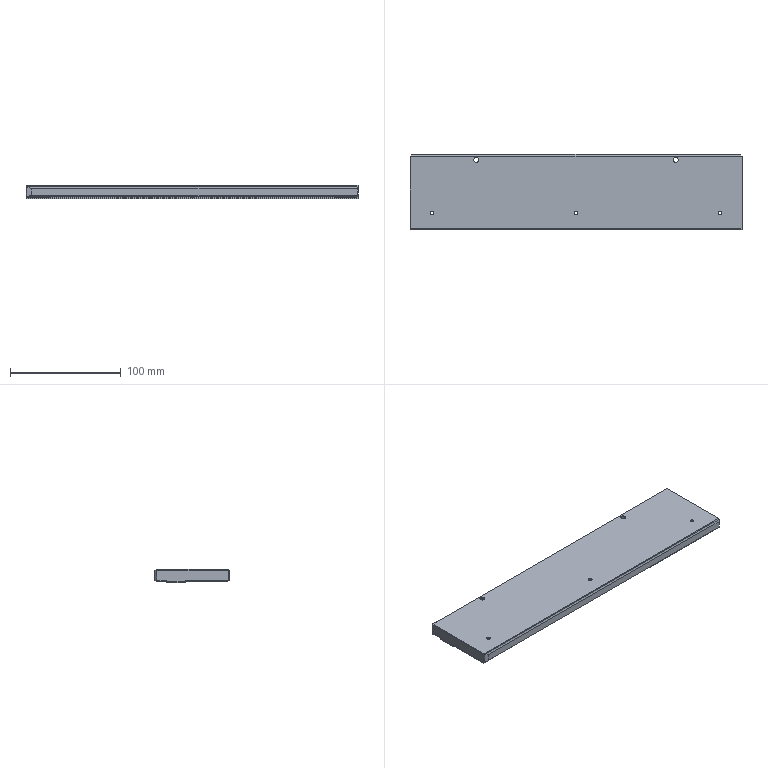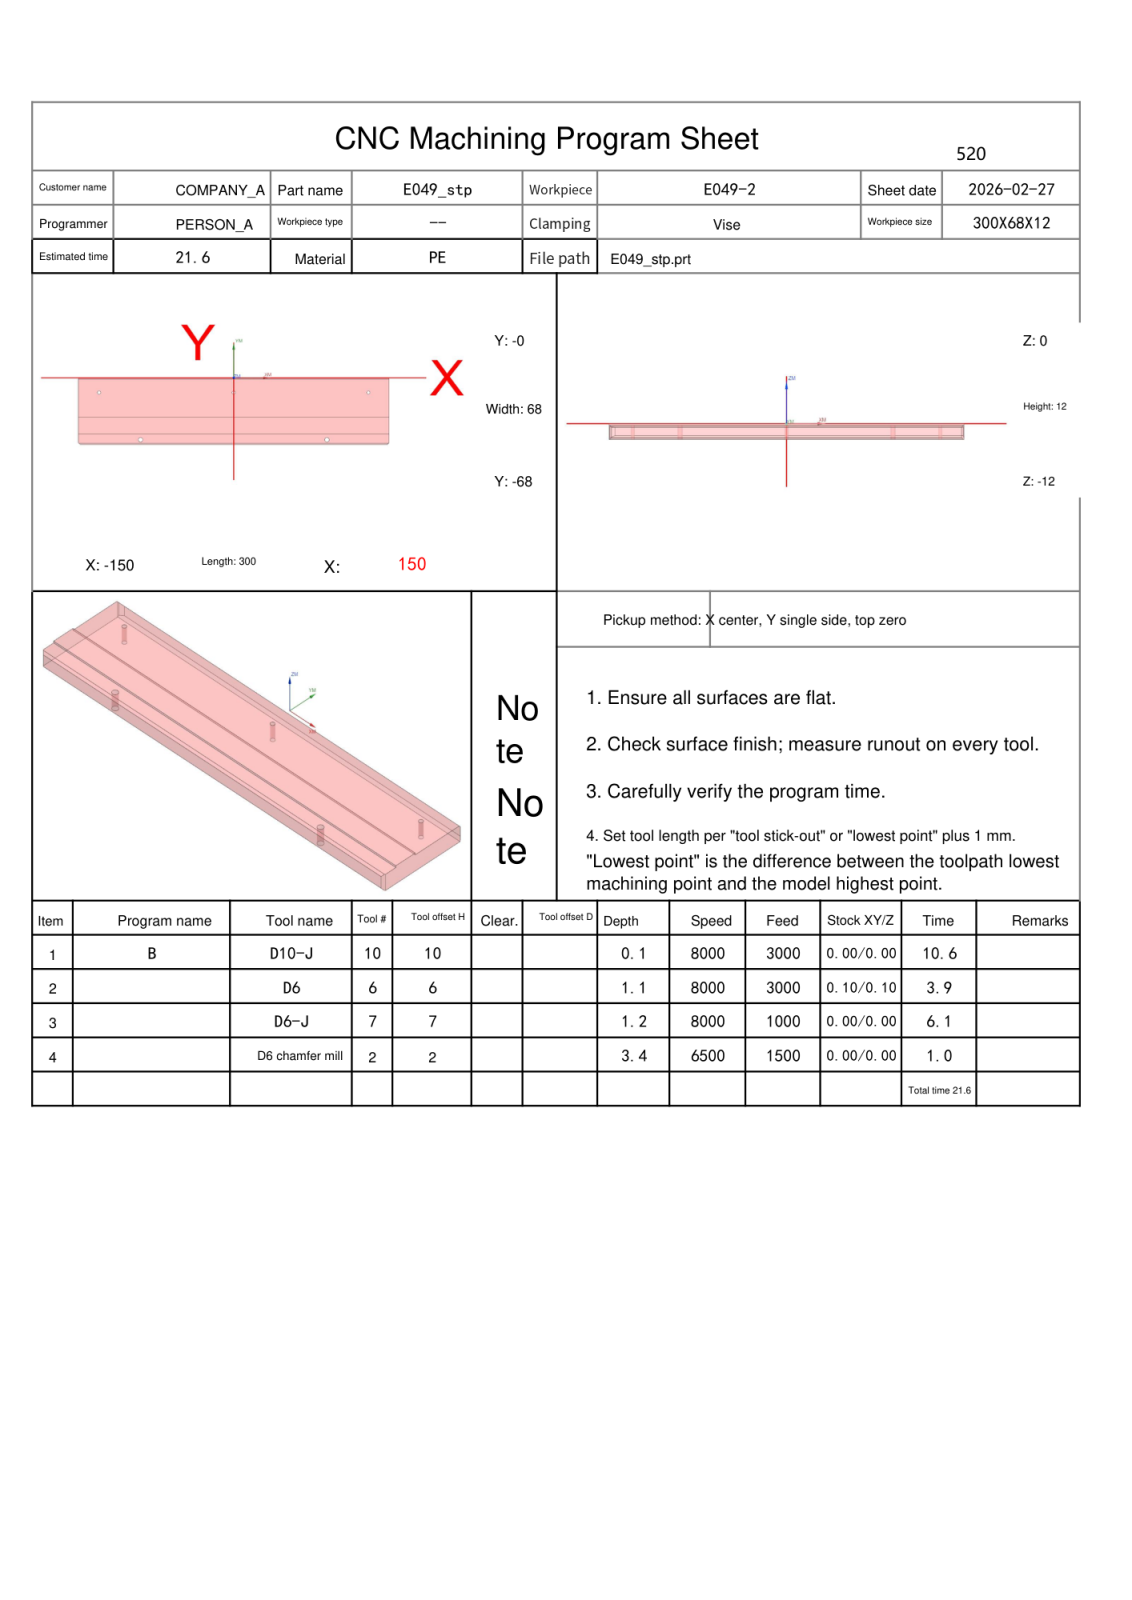NC program | NX | posted by the shop | part box 300 x 68 x 12 mm
Whole program:
%
O0001
(Machine time: 22.30 MIN)
(===Total Tool:4===)
(T10=D10-J  D=10.  R=0.   D-  H10 Z=0.    )
(T6=D6      D=6.   R=0.   D-  H06 Z=-1.1  )
(T7=D6-J    D=6.   R=0.   D7  H07 Z=-1.2  )
(T2=D6 chamfer mill   D=6.   R=0.   D-  H02 Z=-3.4  )
G80 G90 G17 G49 G40
G91 G28 Z0
M01
N1 T10 M06
(D10-J  D=10. R=0. H=10 ce=0.20 di=0.10)
G00 G90 G54 X-167. Y-16.7 M03 S8000
G43 H10 Z50.
M08
Z6.02
G01 Z4.02 F3000.
X-155. Y-4.7
X-145.593 Y4.707
G02 X-144.886 Y5. I.707 J-.707
G01 X-136.565
G02 X-136.166 Y4.6 I0.0 J-.4
X-136.283 Y4.317 I-.4 J0.0
G01 X-154.707 Y-14.107
G03 X-155. Y-14.814 I.707 J-.707
G01 Y-23.135
G03 X-154.6 Y-23.534 I.4 J0.0
X-154.317 Y-23.417 I0.0 J.4
G01 X-126.193 Y4.707
G02 X-125.486 Y5. I.707 J-.707
G01 X-117.165
G02 X-116.766 Y4.6 I0.0 J-.4
X-116.883 Y4.317 I-.4 J0.0
G01 X-154.707 Y-33.507
G03 X-155. Y-34.214 I.707 J-.707
G01 Y-42.535
G03 X-154.6 Y-42.934 I.4 J0.0
X-154.317 Y-42.817 I0.0 J.4
G01 X-106.793 Y4.707
G02 X-106.086 Y5. I.707 J-.707
G01 X-97.765
G02 X-97.366 Y4.6 I0.0 J-.4
X-97.483 Y4.317 I-.4 J0.0
G01 X-154.708 Y-52.908
G03 X-155. Y-53.614 I.708 J-.707
G01 Y-61.935
G03 X-154.6 Y-62.334 I.4 J0.0
X-154.317 Y-62.217 I0.0 J.4
G01 X-87.392 Y4.708
G02 X-86.686 Y5. I.707 J-.708
G01 X-78.365
G02 X-77.966 Y4.6 I0.0 J-.4
X-78.083 Y4.317 I-.4 J0.0
G01 X-154.717 Y-72.317
G03 X-154.834 Y-72.6 I.283 J-.283
X-154.435 Y-73. I.4 J0.0
G01 X-146.114
G03 X-145.408 Y-72.708 I-.001 J1.
G01 X-67.992 Y4.708
G02 X-67.286 Y5. I.707 J-.708
G01 X-58.965
G02 X-58.566 Y4.6 I0.0 J-.4
X-58.683 Y4.317 I-.4 J0.0
G01 X-135.317 Y-72.317
G03 X-135.434 Y-72.6 I.283 J-.283
X-135.035 Y-73. I.4 J0.0
G01 X-126.714
G03 X-126.008 Y-72.708 I-.001 J1.
G01 X-48.592 Y4.708
G02 X-47.886 Y5. I.707 J-.708
G01 X-39.565
G02 X-39.166 Y4.6 I0.0 J-.4
X-39.283 Y4.317 I-.4 J0.0
G01 X-115.917 Y-72.317
G03 X-116.034 Y-72.6 I.283 J-.283
X-115.635 Y-73. I.4 J0.0
G01 X-107.314
G03 X-106.608 Y-72.708 I-.001 J1.
G01 X-29.192 Y4.708
G02 X-28.486 Y5. I.707 J-.708
G01 X-20.165
G02 X-19.766 Y4.6 I0.0 J-.4
X-19.883 Y4.317 I-.4 J0.0
G01 X-96.517 Y-72.317
G03 X-96.634 Y-72.6 I.283 J-.283
X-96.235 Y-73. I.4 J0.0
G01 X-87.914
G03 X-87.208 Y-72.708 I-.001 J1.
G01 X-9.792 Y4.708
G02 X-9.086 Y5. I.707 J-.708
G01 X-.765
G02 X-.366 Y4.6 I0.0 J-.4
X-.483 Y4.317 I-.4 J0.0
G01 X-77.117 Y-72.317
G03 X-77.234 Y-72.6 I.283 J-.283
X-76.835 Y-73. I.4 J0.0
G01 X-68.514
G03 X-67.808 Y-72.708 I-.001 J1.
G01 X9.608 Y4.708
G02 X10.314 Y5. I.707 J-.708
G01 X18.635
G02 X19.034 Y4.6 I0.0 J-.4
X18.917 Y4.317 I-.4 J0.0
G01 X-57.717 Y-72.317
G03 X-57.834 Y-72.6 I.283 J-.283
X-57.435 Y-73. I.4 J0.0
G01 X-49.114
G03 X-48.408 Y-72.708 I-.001 J1.
G01 X29.008 Y4.708
G02 X29.714 Y5. I.707 J-.708
G01 X38.035
G02 X38.434 Y4.6 I0.0 J-.4
X38.317 Y4.317 I-.4 J0.0
G01 X-38.317 Y-72.317
G03 X-38.434 Y-72.6 I.283 J-.283
X-38.035 Y-73. I.4 J0.0
G01 X-29.714
G03 X-29.008 Y-72.708 I-.001 J1.
G01 X48.408 Y4.708
G02 X49.114 Y5. I.707 J-.708
G01 X57.435
G02 X57.834 Y4.6 I0.0 J-.4
X57.717 Y4.317 I-.4 J0.0
G01 X-18.917 Y-72.317
G03 X-19.034 Y-72.6 I.283 J-.283
X-18.635 Y-73. I.4 J0.0
G01 X-10.314
G03 X-9.608 Y-72.708 I-.001 J1.
G01 X67.808 Y4.708
G02 X68.514 Y5. I.707 J-.708
G01 X76.835
G02 X77.234 Y4.6 I0.0 J-.4
X77.117 Y4.317 I-.4 J0.0
G01 X.483 Y-72.317
G03 X.366 Y-72.6 I.283 J-.283
X.765 Y-73. I.4 J0.0
G01 X9.086
G03 X9.792 Y-72.708 I-.001 J1.
G01 X87.208 Y4.708
G02 X87.914 Y5. I.707 J-.708
G01 X96.235
G02 X96.634 Y4.6 I0.0 J-.4
X96.517 Y4.317 I-.4 J0.0
G01 X19.883 Y-72.317
G03 X19.766 Y-72.6 I.283 J-.283
X20.165 Y-73. I.4 J0.0
G01 X28.486
G03 X29.192 Y-72.708 I-.001 J1.
G01 X106.608 Y4.708
G02 X107.314 Y5. I.707 J-.708
G01 X115.635
G02 X116.034 Y4.6 I0.0 J-.4
X115.917 Y4.317 I-.4 J0.0
G01 X39.283 Y-72.317
G03 X39.166 Y-72.6 I.283 J-.283
X39.565 Y-73. I.4 J0.0
G01 X47.886
G03 X48.592 Y-72.708 I-.001 J1.
G01 X126.008 Y4.708
G02 X126.714 Y5. I.707 J-.708
G01 X135.035
G02 X135.434 Y4.6 I0.0 J-.4
X135.317 Y4.317 I-.4 J0.0
G01 X58.683 Y-72.317
G03 X58.566 Y-72.6 I.283 J-.283
X58.965 Y-73. I.4 J0.0
G01 X67.286
G03 X67.992 Y-72.708 I-.001 J1.
G01 X145.408 Y4.708
G02 X146.114 Y5. I.707 J-.708
G01 X154.435
G02 X154.834 Y4.6 I0.0 J-.4
X154.717 Y4.317 I-.4 J0.0
G01 X78.083 Y-72.317
G03 X77.966 Y-72.6 I.283 J-.283
X78.365 Y-73. I.4 J0.0
G01 X86.686
G03 X87.392 Y-72.708 I-.001 J1.
G01 X154.317 Y-5.783
G02 X154.6 Y-5.666 I.283 J-.283
X155. Y-6.065 I0.0 J-.4
G01 Y-14.386
G02 X154.708 Y-15.092 I-1. J.001
G01 X97.483 Y-72.317
G03 X97.366 Y-72.6 I.283 J-.283
X97.765 Y-73. I.4 J0.0
G01 X106.086
G03 X106.792 Y-72.708 I-.001 J1.
G01 X154.317 Y-25.183
G02 X154.6 Y-25.066 I.283 J-.283
X155. Y-25.465 I0.0 J-.4
G01 Y-33.786
G02 X154.707 Y-34.493 I-1. J.001
G01 X116.883 Y-72.317
G03 X116.766 Y-72.6 I.283 J-.283
X117.165 Y-73. I.4 J0.0
G01 X125.486
G03 X126.193 Y-72.707 I0.0 J1.
G01 X154.317 Y-44.583
G02 X154.6 Y-44.466 I.283 J-.283
X155. Y-44.865 I0.0 J-.4
G01 Y-53.186
G02 X154.707 Y-53.893 I-1. J0.0
G01 X136.283 Y-72.317
G03 X136.166 Y-72.6 I.283 J-.283
X136.565 Y-73. I.4 J0.0
G01 X144.886
G03 X145.593 Y-72.707 I0.0 J1.
G01 X155. Y-63.3
X167. Y-51.3
Z6.02
G00 Z8.
X-167. Y-16.7
Z5.04
G01 Z3.04
X-155. Y-4.7
X-145.593 Y4.707
G02 X-144.886 Y5. I.707 J-.707
G01 X-136.565
G02 X-136.166 Y4.6 I0.0 J-.4
X-136.283 Y4.317 I-.4 J0.0
G01 X-154.707 Y-14.107
G03 X-155. Y-14.814 I.707 J-.707
G01 Y-23.135
G03 X-154.6 Y-23.534 I.4 J0.0
X-154.317 Y-23.417 I0.0 J.4
G01 X-126.193 Y4.707
G02 X-125.486 Y5. I.707 J-.707
G01 X-117.165
G02 X-116.766 Y4.6 I0.0 J-.4
X-116.883 Y4.317 I-.4 J0.0
G01 X-154.707 Y-33.507
G03 X-155. Y-34.214 I.707 J-.707
G01 Y-42.535
G03 X-154.6 Y-42.934 I.4 J0.0
X-154.317 Y-42.817 I0.0 J.4
G01 X-106.793 Y4.707
G02 X-106.086 Y5. I.707 J-.707
G01 X-97.765
G02 X-97.366 Y4.6 I0.0 J-.4
X-97.483 Y4.317 I-.4 J0.0
G01 X-154.708 Y-52.908
G03 X-155. Y-53.614 I.708 J-.707
G01 Y-61.935
G03 X-154.6 Y-62.334 I.4 J0.0
X-154.317 Y-62.217 I0.0 J.4
G01 X-87.392 Y4.708
G02 X-86.686 Y5. I.707 J-.708
G01 X-78.365
G02 X-77.966 Y4.6 I0.0 J-.4
X-78.083 Y4.317 I-.4 J0.0
G01 X-154.717 Y-72.317
G03 X-154.834 Y-72.6 I.283 J-.283
X-154.435 Y-73. I.4 J0.0
G01 X-146.114
G03 X-145.408 Y-72.708 I-.001 J1.
G01 X-67.992 Y4.708
G02 X-67.286 Y5. I.707 J-.708
G01 X-58.965
G02 X-58.566 Y4.6 I0.0 J-.4
X-58.683 Y4.317 I-.4 J0.0
G01 X-135.317 Y-72.317
G03 X-135.434 Y-72.6 I.283 J-.283
X-135.035 Y-73. I.4 J0.0
G01 X-126.714
G03 X-126.008 Y-72.708 I-.001 J1.
G01 X-48.592 Y4.708
G02 X-47.886 Y5. I.707 J-.708
G01 X-39.565
G02 X-39.166 Y4.6 I0.0 J-.4
X-39.283 Y4.317 I-.4 J0.0
G01 X-115.917 Y-72.317
G03 X-116.034 Y-72.6 I.283 J-.283
X-115.635 Y-73. I.4 J0.0
G01 X-107.314
G03 X-106.608 Y-72.708 I-.001 J1.
G01 X-29.192 Y4.708
G02 X-28.486 Y5. I.707 J-.708
G01 X-20.165
G02 X-19.766 Y4.6 I0.0 J-.4
X-19.883 Y4.317 I-.4 J0.0
G01 X-96.517 Y-72.317
G03 X-96.634 Y-72.6 I.283 J-.283
X-96.235 Y-73. I.4 J0.0
G01 X-87.914
G03 X-87.208 Y-72.708 I-.001 J1.
G01 X-9.792 Y4.708
G02 X-9.086 Y5. I.707 J-.708
G01 X-.765
G02 X-.366 Y4.6 I0.0 J-.4
X-.483 Y4.317 I-.4 J0.0
G01 X-77.117 Y-72.317
G03 X-77.234 Y-72.6 I.283 J-.283
X-76.835 Y-73. I.4 J0.0
G01 X-68.514
G03 X-67.808 Y-72.708 I-.001 J1.
G01 X9.608 Y4.708
G02 X10.314 Y5. I.707 J-.708
G01 X18.635
G02 X19.034 Y4.6 I0.0 J-.4
X18.917 Y4.317 I-.4 J0.0
G01 X-57.717 Y-72.317
G03 X-57.834 Y-72.6 I.283 J-.283
X-57.435 Y-73. I.4 J0.0
G01 X-49.114
G03 X-48.408 Y-72.708 I-.001 J1.
G01 X29.008 Y4.708
G02 X29.714 Y5. I.707 J-.708
G01 X38.035
G02 X38.434 Y4.6 I0.0 J-.4
X38.317 Y4.317 I-.4 J0.0
G01 X-38.317 Y-72.317
G03 X-38.434 Y-72.6 I.283 J-.283
X-38.035 Y-73. I.4 J0.0
G01 X-29.714
G03 X-29.008 Y-72.708 I-.001 J1.
G01 X48.408 Y4.708
G02 X49.114 Y5. I.707 J-.708
G01 X57.435
G02 X57.834 Y4.6 I0.0 J-.4
X57.717 Y4.317 I-.4 J0.0
G01 X-18.917 Y-72.317
G03 X-19.034 Y-72.6 I.283 J-.283
X-18.635 Y-73. I.4 J0.0
G01 X-10.314
G03 X-9.608 Y-72.708 I-.001 J1.
G01 X67.808 Y4.708
G02 X68.514 Y5. I.707 J-.708
G01 X76.835
G02 X77.234 Y4.6 I0.0 J-.4
X77.117 Y4.317 I-.4 J0.0
G01 X.483 Y-72.317
G03 X.366 Y-72.6 I.283 J-.283
X.765 Y-73. I.4 J0.0
G01 X9.086
G03 X9.792 Y-72.708 I-.001 J1.
G01 X87.208 Y4.708
G02 X87.914 Y5. I.707 J-.708
G01 X96.235
G02 X96.634 Y4.6 I0.0 J-.4
X96.517 Y4.317 I-.4 J0.0
G01 X19.883 Y-72.317
G03 X19.766 Y-72.6 I.283 J-.283
X20.165 Y-73. I.4 J0.0
G01 X28.486
G03 X29.192 Y-72.708 I-.001 J1.
G01 X106.608 Y4.708
G02 X107.314 Y5. I.707 J-.708
G01 X115.635
G02 X116.034 Y4.6 I0.0 J-.4
X115.917 Y4.317 I-.4 J0.0
G01 X39.283 Y-72.317
G03 X39.166 Y-72.6 I.283 J-.283
X39.565 Y-73. I.4 J0.0
G01 X47.886
G03 X48.592 Y-72.708 I-.001 J1.
G01 X126.008 Y4.708
G02 X126.714 Y5. I.707 J-.708
G01 X135.035
G02 X135.434 Y4.6 I0.0 J-.4
X135.317 Y4.317 I-.4 J0.0
G01 X58.683 Y-72.317
G03 X58.566 Y-72.6 I.283 J-.283
X58.965 Y-73. I.4 J0.0
G01 X67.286
G03 X67.992 Y-72.708 I-.001 J1.
G01 X145.408 Y4.708
G02 X146.114 Y5. I.707 J-.708
G01 X154.435
G02 X154.834 Y4.6 I0.0 J-.4
X154.717 Y4.317 I-.4 J0.0
G01 X78.083 Y-72.317
G03 X77.966 Y-72.6 I.283 J-.283
X78.365 Y-73. I.4 J0.0
G01 X86.686
G03 X87.392 Y-72.708 I-.001 J1.
G01 X154.317 Y-5.783
G02 X154.6 Y-5.666 I.283 J-.283
X155. Y-6.065 I0.0 J-.4
G01 Y-14.386
G02 X154.708 Y-15.092 I-1. J.001
G01 X97.483 Y-72.317
G03 X97.366 Y-72.6 I.283 J-.283
X97.765 Y-73. I.4 J0.0
G01 X106.086
G03 X106.792 Y-72.708 I-.001 J1.
G01 X154.317 Y-25.183
G02 X154.6 Y-25.066 I.283 J-.283
X155. Y-25.465 I0.0 J-.4
G01 Y-33.786
G02 X154.707 Y-34.493 I-1. J.001
G01 X116.883 Y-72.317
G03 X116.766 Y-72.6 I.283 J-.283
X117.165 Y-73. I.4 J0.0
G01 X125.486
G03 X126.193 Y-72.707 I0.0 J1.
G01 X154.317 Y-44.583
G02 X154.6 Y-44.466 I.283 J-.283
X155. Y-44.865 I0.0 J-.4
G01 Y-53.186
G02 X154.707 Y-53.893 I-1. J0.0
G01 X136.283 Y-72.317
G03 X136.166 Y-72.6 I.283 J-.283
X136.565 Y-73. I.4 J0.0
G01 X144.886
G03 X145.593 Y-72.707 I0.0 J1.
G01 X155. Y-63.3
X167. Y-51.3
Z5.04
G00 Z7.02
X-167. Y-16.7
Z4.06
G01 Z2.06
X-155. Y-4.7
X-145.593 Y4.707
G02 X-144.886 Y5. I.707 J-.707
G01 X-136.565
G02 X-136.166 Y4.6 I0.0 J-.4
X-136.283 Y4.317 I-.4 J0.0
G01 X-154.707 Y-14.107
G03 X-155. Y-14.814 I.707 J-.707
G01 Y-23.135
G03 X-154.6 Y-23.534 I.4 J0.0
X-154.317 Y-23.417 I0.0 J.4
G01 X-126.193 Y4.707
G02 X-125.486 Y5. I.707 J-.707
G01 X-117.165
G02 X-116.766 Y4.6 I0.0 J-.4
X-116.883 Y4.317 I-.4 J0.0
G01 X-154.707 Y-33.507
G03 X-155. Y-34.214 I.707 J-.707
G01 Y-42.535
G03 X-154.6 Y-42.934 I.4 J0.0
X-154.317 Y-42.817 I0.0 J.4
G01 X-106.793 Y4.707
G02 X-106.086 Y5. I.707 J-.707
G01 X-97.765
G02 X-97.366 Y4.6 I0.0 J-.4
X-97.483 Y4.317 I-.4 J0.0
G01 X-154.708 Y-52.908
G03 X-155. Y-53.614 I.708 J-.707
G01 Y-61.935
G03 X-154.6 Y-62.334 I.4 J0.0
X-154.317 Y-62.217 I0.0 J.4
G01 X-87.392 Y4.708
G02 X-86.686 Y5. I.707 J-.708
G01 X-78.365
G02 X-77.966 Y4.6 I0.0 J-.4
X-78.083 Y4.317 I-.4 J0.0
G01 X-154.717 Y-72.317
G03 X-154.834 Y-72.6 I.283 J-.283
X-154.435 Y-73. I.4 J0.0
G01 X-146.114
G03 X-145.408 Y-72.708 I-.001 J1.
G01 X-67.992 Y4.708
G02 X-67.286 Y5. I.707 J-.708
G01 X-58.965
G02 X-58.566 Y4.6 I0.0 J-.4
X-58.683 Y4.317 I-.4 J0.0
G01 X-135.317 Y-72.317
G03 X-135.434 Y-72.6 I.283 J-.283
X-135.035 Y-73. I.4 J0.0
G01 X-126.714
G03 X-126.008 Y-72.708 I-.001 J1.
G01 X-48.592 Y4.708
G02 X-47.886 Y5. I.707 J-.708
G01 X-39.565
G02 X-39.166 Y4.6 I0.0 J-.4
X-39.283 Y4.317 I-.4 J0.0
G01 X-115.917 Y-72.317
G03 X-116.034 Y-72.6 I.283 J-.283
X-115.635 Y-73. I.4 J0.0
G01 X-107.314
G03 X-106.608 Y-72.708 I-.001 J1.
G01 X-29.192 Y4.708
G02 X-28.486 Y5. I.707 J-.708
G01 X-20.165
G02 X-19.766 Y4.6 I0.0 J-.4
X-19.883 Y4.317 I-.4 J0.0
G01 X-96.517 Y-72.317
G03 X-96.634 Y-72.6 I.283 J-.283
X-96.235 Y-73. I.4 J0.0
G01 X-87.914
G03 X-87.208 Y-72.708 I-.001 J1.
G01 X-9.792 Y4.708
G02 X-9.086 Y5. I.707 J-.708
G01 X-.765
G02 X-.366 Y4.6 I0.0 J-.4
X-.483 Y4.317 I-.4 J0.0
G01 X-77.117 Y-72.317
G03 X-77.234 Y-72.6 I.283 J-.283
X-76.835 Y-73. I.4 J0.0
G01 X-68.514
G03 X-67.808 Y-72.708 I-.001 J1.
G01 X9.608 Y4.708
G02 X10.314 Y5. I.707 J-.708
G01 X18.635
G02 X19.034 Y4.6 I0.0 J-.4
X18.917 Y4.317 I-.4 J0.0
G01 X-57.717 Y-72.317
G03 X-57.834 Y-72.6 I.283 J-.283
X-57.435 Y-73. I.4 J0.0
G01 X-49.114
G03 X-48.408 Y-72.708 I-.001 J1.
G01 X29.008 Y4.708
G02 X29.714 Y5. I.707 J-.708
G01 X38.035
G02 X38.434 Y4.6 I0.0 J-.4
X38.317 Y4.317 I-.4 J0.0
G01 X-38.317 Y-72.317
G03 X-38.434 Y-72.6 I.283 J-.283
X-38.035 Y-73. I.4 J0.0
G01 X-29.714
G03 X-29.008 Y-72.708 I-.001 J1.
G01 X48.408 Y4.708
G02 X49.114 Y5. I.707 J-.708
G01 X57.435
G02 X57.834 Y4.6 I0.0 J-.4
X57.717 Y4.317 I-.4 J0.0
G01 X-18.917 Y-72.317
G03 X-19.034 Y-72.6 I.283 J-.283
X-18.635 Y-73. I.4 J0.0
G01 X-10.314
G03 X-9.608 Y-72.708 I-.001 J1.
G01 X67.808 Y4.708
G02 X68.514 Y5. I.707 J-.708
G01 X76.835
G02 X77.234 Y4.6 I0.0 J-.4
X77.117 Y4.317 I-.4 J0.0
G01 X.483 Y-72.317
G03 X.366 Y-72.6 I.283 J-.283
X.765 Y-73. I.4 J0.0
G01 X9.086
G03 X9.792 Y-72.708 I-.001 J1.
G01 X87.208 Y4.708
G02 X87.914 Y5. I.707 J-.708
G01 X96.235
G02 X96.634 Y4.6 I0.0 J-.4
X96.517 Y4.317 I-.4 J0.0
G01 X19.883 Y-72.317
G03 X19.766 Y-72.6 I.283 J-.283
X20.165 Y-73. I.4 J0.0
G01 X28.486
G03 X29.192 Y-72.708 I-.001 J1.
G01 X106.608 Y4.708
G02 X107.314 Y5. I.707 J-.708
G01 X115.635
G02 X116.034 Y4.6 I0.0 J-.4
X115.917 Y4.317 I-.4 J0.0
G01 X39.283 Y-72.317
G03 X39.166 Y-72.6 I.283 J-.283
X39.565 Y-73. I.4 J0.0
G01 X47.886
G03 X48.592 Y-72.708 I-.001 J1.
G01 X126.008 Y4.708
G02 X126.714 Y5. I.707 J-.708
G01 X135.035
G02 X135.434 Y4.6 I0.0 J-.4
X135.317 Y4.317 I-.4 J0.0
G01 X58.683 Y-72.317
G03 X58.566 Y-72.6 I.283 J-.283
X58.965 Y-73. I.4 J0.0
G01 X67.286
G03 X67.992 Y-72.708 I-.001 J1.
G01 X145.408 Y4.708
G02 X146.114 Y5. I.707 J-.708
G01 X154.435
G02 X154.834 Y4.6 I0.0 J-.4
X154.717 Y4.317 I-.4 J0.0
G01 X78.083 Y-72.317
G03 X77.966 Y-72.6 I.283 J-.283
X78.365 Y-73. I.4 J0.0
G01 X86.686
G03 X87.392 Y-72.708 I-.001 J1.
G01 X154.317 Y-5.783
G02 X154.6 Y-5.666 I.283 J-.283
X155. Y-6.065 I0.0 J-.4
G01 Y-14.386
G02 X154.708 Y-15.092 I-1. J.001
G01 X97.483 Y-72.317
G03 X97.366 Y-72.6 I.283 J-.283
X97.765 Y-73. I.4 J0.0
G01 X106.086
G03 X106.792 Y-72.708 I-.001 J1.
G01 X154.317 Y-25.183
G02 X154.6 Y-25.066 I.283 J-.283
X155. Y-25.465 I0.0 J-.4
G01 Y-33.786
G02 X154.707 Y-34.493 I-1. J.001
G01 X116.883 Y-72.317
G03 X116.766 Y-72.6 I.283 J-.283
X117.165 Y-73. I.4 J0.0
G01 X125.486
G03 X126.193 Y-72.707 I0.0 J1.
G01 X154.317 Y-44.583
G02 X154.6 Y-44.466 I.283 J-.283
X155. Y-44.865 I0.0 J-.4
G01 Y-53.186
G02 X154.707 Y-53.893 I-1. J0.0
G01 X136.283 Y-72.317
G03 X136.166 Y-72.6 I.283 J-.283
X136.565 Y-73. I.4 J0.0
G01 X144.886
G03 X145.593 Y-72.707 I0.0 J1.
G01 X155. Y-63.3
X167. Y-51.3
Z4.06
G00 Z6.04
X-167. Y-16.7
Z3.08
G01 Z1.08
X-155. Y-4.7
X-145.593 Y4.707
G02 X-144.886 Y5. I.707 J-.707
G01 X-136.565
G02 X-136.166 Y4.6 I0.0 J-.4
X-136.283 Y4.317 I-.4 J0.0
G01 X-154.707 Y-14.107
G03 X-155. Y-14.814 I.707 J-.707
G01 Y-23.135
G03 X-154.6 Y-23.534 I.4 J0.0
X-154.317 Y-23.417 I0.0 J.4
G01 X-126.193 Y4.707
G02 X-125.486 Y5. I.707 J-.707
G01 X-117.165
G02 X-116.766 Y4.6 I0.0 J-.4
X-116.883 Y4.317 I-.4 J0.0
G01 X-154.707 Y-33.507
G03 X-155. Y-34.214 I.707 J-.707
G01 Y-42.535
G03 X-154.6 Y-42.934 I.4 J0.0
X-154.317 Y-42.817 I0.0 J.4
G01 X-106.793 Y4.707
G02 X-106.086 Y5. I.707 J-.707
G01 X-97.765
G02 X-97.366 Y4.6 I0.0 J-.4
X-97.483 Y4.317 I-.4 J0.0
G01 X-154.708 Y-52.908
G03 X-155. Y-53.614 I.708 J-.707
G01 Y-61.935
G03 X-154.6 Y-62.334 I.4 J0.0
X-154.317 Y-62.217 I0.0 J.4
G01 X-87.392 Y4.708
G02 X-86.686 Y5. I.707 J-.708
G01 X-78.365
G02 X-77.966 Y4.6 I0.0 J-.4
X-78.083 Y4.317 I-.4 J0.0
G01 X-154.717 Y-72.317
G03 X-154.834 Y-72.6 I.283 J-.283
X-154.435 Y-73. I.4 J0.0
G01 X-146.114
G03 X-145.408 Y-72.708 I-.001 J1.
G01 X-67.992 Y4.708
G02 X-67.286 Y5. I.707 J-.708
G01 X-58.965
G02 X-58.566 Y4.6 I0.0 J-.4
X-58.683 Y4.317 I-.4 J0.0
G01 X-135.317 Y-72.317
G03 X-135.434 Y-72.6 I.283 J-.283
X-135.035 Y-73. I.4 J0.0
G01 X-126.714
G03 X-126.008 Y-72.708 I-.001 J1.
G01 X-48.592 Y4.708
G02 X-47.886 Y5. I.707 J-.708
G01 X-39.565
G02 X-39.166 Y4.6 I0.0 J-.4
X-39.283 Y4.317 I-.4 J0.0
G01 X-115.917 Y-72.317
G03 X-116.034 Y-72.6 I.283 J-.283
X-115.635 Y-73. I.4 J0.0
G01 X-107.314
G03 X-106.608 Y-72.708 I-.001 J1.
G01 X-29.192 Y4.708
G02 X-28.486 Y5. I.707 J-.708
G01 X-20.165
G02 X-19.766 Y4.6 I0.0 J-.4
X-19.883 Y4.317 I-.4 J0.0
G01 X-96.517 Y-72.317
G03 X-96.634 Y-72.6 I.283 J-.283
X-96.235 Y-73. I.4 J0.0
G01 X-87.914
G03 X-87.208 Y-72.708 I-.001 J1.
G01 X-9.792 Y4.708
G02 X-9.086 Y5. I.707 J-.708
G01 X-.765
G02 X-.366 Y4.6 I0.0 J-.4
X-.483 Y4.317 I-.4 J0.0
G01 X-77.117 Y-72.317
G03 X-77.234 Y-72.6 I.283 J-.283
X-76.835 Y-73. I.4 J0.0
G01 X-68.514
G03 X-67.808 Y-72.708 I-.001 J1.
G01 X9.608 Y4.708
G02 X10.314 Y5. I.707 J-.708
G01 X18.635
G02 X19.034 Y4.6 I0.0 J-.4
X18.917 Y4.317 I-.4 J0.0
G01 X-57.717 Y-72.317
G03 X-57.834 Y-72.6 I.283 J-.283
X-57.435 Y-73. I.4 J0.0
G01 X-49.114
G03 X-48.408 Y-72.708 I-.001 J1.
G01 X29.008 Y4.708
G02 X29.714 Y5. I.707 J-.708
G01 X38.035
G02 X38.434 Y4.6 I0.0 J-.4
X38.317 Y4.317 I-.4 J0.0
G01 X-38.317 Y-72.317
G03 X-38.434 Y-72.6 I.283 J-.283
X-38.035 Y-73. I.4 J0.0
G01 X-29.714
G03 X-29.008 Y-72.708 I-.001 J1.
G01 X48.408 Y4.708
G02 X49.114 Y5. I.707 J-.708
G01 X57.435
G02 X57.834 Y4.6 I0.0 J-.4
X57.717 Y4.317 I-.4 J0.0
G01 X-18.917 Y-72.317
G03 X-19.034 Y-72.6 I.283 J-.283
X-18.635 Y-73. I.4 J0.0
G01 X-10.314
G03 X-9.608 Y-72.708 I-.001 J1.
G01 X67.808 Y4.708
G02 X68.514 Y5. I.707 J-.708
G01 X76.835
G02 X77.234 Y4.6 I0.0 J-.4
X77.117 Y4.317 I-.4 J0.0
G01 X.483 Y-72.317
G03 X.366 Y-72.6 I.283 J-.283
X.765 Y-73. I.4 J0.0
G01 X9.086
G03 X9.792 Y-72.708 I-.001 J1.
G01 X87.208 Y4.708
G02 X87.914 Y5. I.707 J-.708
G01 X96.235
G02 X96.634 Y4.6 I0.0 J-.4
X96.517 Y4.317 I-.4 J0.0
G01 X19.883 Y-72.317
G03 X19.766 Y-72.6 I.283 J-.283
X20.165 Y-73. I.4 J0.0
G01 X28.486
G03 X29.192 Y-72.708 I-.001 J1.
G01 X106.608 Y4.708
G02 X107.314 Y5. I.707 J-.708
G01 X115.635
G02 X116.034 Y4.6 I0.0 J-.4
X115.917 Y4.317 I-.4 J0.0
G01 X39.283 Y-72.317
G03 X39.166 Y-72.6 I.283 J-.283
X39.565 Y-73. I.4 J0.0
G01 X47.886
G03 X48.592 Y-72.708 I-.001 J1.
G01 X126.008 Y4.708
G02 X126.714 Y5. I.707 J-.708
G01 X135.035
G02 X135.434 Y4.6 I0.0 J-.4
X135.317 Y4.317 I-.4 J0.0
G01 X58.683 Y-72.317
G03 X58.566 Y-72.6 I.283 J-.283
X58.965 Y-73. I.4 J0.0
G01 X67.286
G03 X67.992 Y-72.708 I-.001 J1.
G01 X145.408 Y4.708
G02 X146.114 Y5. I.707 J-.708
G01 X154.435
G02 X154.834 Y4.6 I0.0 J-.4
X154.717 Y4.317 I-.4 J0.0
G01 X78.083 Y-72.317
G03 X77.966 Y-72.6 I.283 J-.283
X78.365 Y-73. I.4 J0.0
G01 X86.686
G03 X87.392 Y-72.708 I-.001 J1.
G01 X154.317 Y-5.783
G02 X154.6 Y-5.666 I.283 J-.283
X155. Y-6.065 I0.0 J-.4
G01 Y-14.386
G02 X154.708 Y-15.092 I-1. J.001
G01 X97.483 Y-72.317
G03 X97.366 Y-72.6 I.283 J-.283
X97.765 Y-73. I.4 J0.0
G01 X106.086
G03 X106.792 Y-72.708 I-.001 J1.
G01 X154.317 Y-25.183
G02 X154.6 Y-25.066 I.283 J-.283
X155. Y-25.465 I0.0 J-.4
G01 Y-33.786
G02 X154.707 Y-34.493 I-1. J.001
G01 X116.883 Y-72.317
G03 X116.766 Y-72.6 I.283 J-.283
X117.165 Y-73. I.4 J0.0
G01 X125.486
G03 X126.193 Y-72.707 I0.0 J1.
G01 X154.317 Y-44.583
G02 X154.6 Y-44.466 I.283 J-.283
X155. Y-44.865 I0.0 J-.4
G01 Y-53.186
G02 X154.707 Y-53.893 I-1. J0.0
G01 X136.283 Y-72.317
G03 X136.166 Y-72.6 I.283 J-.283
X136.565 Y-73. I.4 J0.0
G01 X144.886
G03 X145.593 Y-72.707 I0.0 J1.
G01 X155. Y-63.3
X167. Y-51.3
Z3.08
G00 Z5.06
X-167. Y-16.7
Z2.1
G01 Z.1
X-155. Y-4.7
X-145.593 Y4.707
G02 X-144.886 Y5. I.707 J-.707
G01 X-136.565
G02 X-136.166 Y4.6 I0.0 J-.4
X-136.283 Y4.317 I-.4 J0.0
G01 X-154.707 Y-14.107
G03 X-155. Y-14.814 I.707 J-.707
G01 Y-23.135
G03 X-154.6 Y-23.534 I.4 J0.0
X-154.317 Y-23.417 I0.0 J.4
G01 X-126.193 Y4.707
G02 X-125.486 Y5. I.707 J-.707
G01 X-117.165
G02 X-116.766 Y4.6 I0.0 J-.4
X-116.883 Y4.317 I-.4 J0.0
G01 X-154.707 Y-33.507
G03 X-155. Y-34.214 I.707 J-.707
G01 Y-42.535
G03 X-154.6 Y-42.934 I.4 J0.0
X-154.317 Y-42.817 I0.0 J.4
G01 X-106.793 Y4.707
G02 X-106.086 Y5. I.707 J-.707
G01 X-97.765
G02 X-97.366 Y4.6 I0.0 J-.4
X-97.483 Y4.317 I-.4 J0.0
G01 X-154.708 Y-52.908
G03 X-155. Y-53.614 I.708 J-.707
G01 Y-61.935
G03 X-154.6 Y-62.334 I.4 J0.0
X-154.317 Y-62.217 I0.0 J.4
G01 X-87.392 Y4.708
G02 X-86.686 Y5. I.707 J-.708
G01 X-78.365
G02 X-77.966 Y4.6 I0.0 J-.4
X-78.083 Y4.317 I-.4 J0.0
G01 X-154.717 Y-72.317
G03 X-154.834 Y-72.6 I.283 J-.283
X-154.435 Y-73. I.4 J0.0
G01 X-146.114
G03 X-145.408 Y-72.708 I-.001 J1.
G01 X-67.992 Y4.708
G02 X-67.286 Y5. I.707 J-.708
G01 X-58.965
G02 X-58.566 Y4.6 I0.0 J-.4
X-58.683 Y4.317 I-.4 J0.0
G01 X-135.317 Y-72.317
G03 X-135.434 Y-72.6 I.283 J-.283
X-135.035 Y-73. I.4 J0.0
G01 X-126.714
G03 X-126.008 Y-72.708 I-.001 J1.
G01 X-48.592 Y4.708
G02 X-47.886 Y5. I.707 J-.708
G01 X-39.565
G02 X-39.166 Y4.6 I0.0 J-.4
X-39.283 Y4.317 I-.4 J0.0
G01 X-115.917 Y-72.317
G03 X-116.034 Y-72.6 I.283 J-.283
X-115.635 Y-73. I.4 J0.0
G01 X-107.314
G03 X-106.608 Y-72.708 I-.001 J1.
G01 X-29.192 Y4.708
G02 X-28.486 Y5. I.707 J-.708
G01 X-20.165
G02 X-19.766 Y4.6 I0.0 J-.4
X-19.883 Y4.317 I-.4 J0.0
G01 X-96.517 Y-72.317
G03 X-96.634 Y-72.6 I.283 J-.283
X-96.235 Y-73. I.4 J0.0
G01 X-87.914
G03 X-87.208 Y-72.708 I-.001 J1.
G01 X-9.792 Y4.708
G02 X-9.086 Y5. I.707 J-.708
G01 X-.765
G02 X-.366 Y4.6 I0.0 J-.4
X-.483 Y4.317 I-.4 J0.0
G01 X-77.117 Y-72.317
G03 X-77.234 Y-72.6 I.283 J-.283
X-76.835 Y-73. I.4 J0.0
G01 X-68.514
G03 X-67.808 Y-72.708 I-.001 J1.
G01 X9.608 Y4.708
G02 X10.314 Y5. I.707 J-.708
G01 X18.635
G02 X19.034 Y4.6 I0.0 J-.4
X18.917 Y4.317 I-.4 J0.0
G01 X-57.717 Y-72.317
G03 X-57.834 Y-72.6 I.283 J-.283
X-57.435 Y-73. I.4 J0.0
G01 X-49.114
G03 X-48.408 Y-72.708 I-.001 J1.
G01 X29.008 Y4.708
G02 X29.714 Y5. I.707 J-.708
G01 X38.035
G02 X38.434 Y4.6 I0.0 J-.4
X38.317 Y4.317 I-.4 J0.0
G01 X-38.317 Y-72.317
G03 X-38.434 Y-72.6 I.283 J-.283
X-38.035 Y-73. I.4 J0.0
G01 X-29.714
G03 X-29.008 Y-72.708 I-.001 J1.
G01 X48.408 Y4.708
G02 X49.114 Y5. I.707 J-.708
G01 X57.435
G02 X57.834 Y4.6 I0.0 J-.4
X57.717 Y4.317 I-.4 J0.0
G01 X-18.917 Y-72.317
G03 X-19.034 Y-72.6 I.283 J-.283
X-18.635 Y-73. I.4 J0.0
G01 X-10.314
G03 X-9.608 Y-72.708 I-.001 J1.
G01 X67.808 Y4.708
G02 X68.514 Y5. I.707 J-.708
G01 X76.835
G02 X77.234 Y4.6 I0.0 J-.4
X77.117 Y4.317 I-.4 J0.0
G01 X.483 Y-72.317
G03 X.366 Y-72.6 I.283 J-.283
X.765 Y-73. I.4 J0.0
G01 X9.086
G03 X9.792 Y-72.708 I-.001 J1.
G01 X87.208 Y4.708
G02 X87.914 Y5. I.707 J-.708
G01 X96.235
G02 X96.634 Y4.6 I0.0 J-.4
X96.517 Y4.317 I-.4 J0.0
G01 X19.883 Y-72.317
G03 X19.766 Y-72.6 I.283 J-.283
X20.165 Y-73. I.4 J0.0
G01 X28.486
G03 X29.192 Y-72.708 I-.001 J1.
G01 X106.608 Y4.708
G02 X107.314 Y5. I.707 J-.708
G01 X115.635
G02 X116.034 Y4.6 I0.0 J-.4
X115.917 Y4.317 I-.4 J0.0
G01 X39.283 Y-72.317
G03 X39.166 Y-72.6 I.283 J-.283
X39.565 Y-73. I.4 J0.0
G01 X47.886
G03 X48.592 Y-72.708 I-.001 J1.
G01 X126.008 Y4.708
G02 X126.714 Y5. I.707 J-.708
G01 X135.035
G02 X135.434 Y4.6 I0.0 J-.4
X135.317 Y4.317 I-.4 J0.0
G01 X58.683 Y-72.317
G03 X58.566 Y-72.6 I.283 J-.283
X58.965 Y-73. I.4 J0.0
G01 X67.286
G03 X67.992 Y-72.708 I-.001 J1.
G01 X145.408 Y4.708
G02 X146.114 Y5. I.707 J-.708
G01 X154.435
G02 X154.834 Y4.6 I0.0 J-.4
X154.717 Y4.317 I-.4 J0.0
G01 X78.083 Y-72.317
G03 X77.966 Y-72.6 I.283 J-.283
X78.365 Y-73. I.4 J0.0
G01 X86.686
G03 X87.392 Y-72.708 I-.001 J1.
G01 X154.317 Y-5.783
G02 X154.6 Y-5.666 I.283 J-.283
X155. Y-6.065 I0.0 J-.4
G01 Y-14.386
G02 X154.708 Y-15.092 I-1. J.001
G01 X97.483 Y-72.317
G03 X97.366 Y-72.6 I.283 J-.283
X97.765 Y-73. I.4 J0.0
G01 X106.086
G03 X106.792 Y-72.708 I-.001 J1.
G01 X154.317 Y-25.183
G02 X154.6 Y-25.066 I.283 J-.283
X155. Y-25.465 I0.0 J-.4
G01 Y-33.786
G02 X154.707 Y-34.493 I-1. J.001
G01 X116.883 Y-72.317
G03 X116.766 Y-72.6 I.283 J-.283
X117.165 Y-73. I.4 J0.0
G01 X125.486
G03 X126.193 Y-72.707 I0.0 J1.
G01 X154.317 Y-44.583
G02 X154.6 Y-44.466 I.283 J-.283
X155. Y-44.865 I0.0 J-.4
G01 Y-53.186
G02 X154.707 Y-53.893 I-1. J0.0
G01 X136.283 Y-72.317
G03 X136.166 Y-72.6 I.283 J-.283
X136.565 Y-73. I.4 J0.0
G01 X144.886
G03 X145.593 Y-72.707 I0.0 J1.
G01 X155. Y-63.3
X167. Y-51.3
Z2.1
G00 Z50.
G00 G90 X-167. Y-16.7 M03 S8000
Z50.
Z2.
G01 Z0.0 F1000.
X-155. Y-4.7
X-145.3 Y5.
X-135.6
X-155. Y-14.4
Y-24.1
X-125.9 Y5.
X-116.2
X-155. Y-33.8
Y-43.5
X-106.5 Y5.
X-96.8
X-155. Y-53.2
Y-62.9
X-87.1 Y5.
X-77.4
X-155. Y-72.6
Y-73.
X-145.7
X-67.7 Y5.
X-58.
X-136. Y-73.
X-126.3
X-48.3 Y5.
X-38.6
X-116.6 Y-73.
X-106.9
X-28.9 Y5.
X-19.2
X-97.2 Y-73.
X-87.5
X-9.5 Y5.
X.2
X-77.8 Y-73.
X-68.1
X9.9 Y5.
X19.6
X-58.4 Y-73.
X-48.7
X29.3 Y5.
X39.
X-39. Y-73.
X-29.3
X48.7 Y5.
X58.4
X-19.6 Y-73.
X-9.9
X68.1 Y5.
X77.8
X-.2 Y-73.
X9.5
X87.5 Y5.
X97.2
X19.2 Y-73.
X28.9
X106.9 Y5.
X116.6
X38.6 Y-73.
X48.3
X126.3 Y5.
X136.
X58. Y-73.
X67.7
X145.7 Y5.
X155.
Y4.6
X77.4 Y-73.
X87.1
X155. Y-5.1
Y-14.8
X96.8 Y-73.
X106.5
X155. Y-24.5
Y-34.2
X116.2 Y-73.
X125.9
X155. Y-43.9
Y-53.6
X135.6 Y-73.
X145.3
X155. Y-63.3
X167. Y-51.3
Z2.
G00 Z50.
G91 G28 Z0.0
M05
M09
G91 G28 Z0.0
M01
N2 T06 M06
(D6  D=6. R=0. H=06 ce=0.10 di=0.10)
G00 G90 G54 X155.353 Y-69.1 M03 S8000
G43 H06 Z12.5
M08
Z1.133
G01 Z-.367 F3000.
X151.058
X-150.81
G02 X-151.233 Y-68.925 I.001 J.6
G01 X-152.764 Y-67.393
G02 X-152.94 Y-66.969 I.424 J.424
G01 Y-65.199
G02 X-152.341 Y-64.6 I.6 J-.001
G01 X152.427
G03 X153.019 Y-64.093 I-.001 J.6
G01 X153.533 Y-60.792
X153.54 Y-60.7
G03 X152.94 Y-60.1 I-.6 J0.0
G01 X-152.94
X-156.1
Z1.133
G00 X155.353 Y-69.1
Z.767
G01 Z-.733
X151.058
X-150.81
G02 X-151.233 Y-68.925 I.001 J.6
G01 X-152.764 Y-67.393
G02 X-152.94 Y-66.969 I.424 J.424
G01 Y-65.199
G02 X-152.341 Y-64.6 I.6 J-.001
G01 X152.427
G03 X153.019 Y-64.093 I-.001 J.6
G01 X153.533 Y-60.792
X153.54 Y-60.7
G03 X152.94 Y-60.1 I-.6 J0.0
G01 X-152.94
X-156.1
Z.767
G00 X155.353 Y-69.1
Z.4
G01 Z-1.1
X151.058
X-150.81
G02 X-151.233 Y-68.925 I.001 J.6
G01 X-152.764 Y-67.393
G02 X-152.94 Y-66.969 I.424 J.424
G01 Y-65.199
G02 X-152.341 Y-64.6 I.6 J-.001
G01 X152.427
G03 X153.019 Y-64.093 I-.001 J.6
G01 X153.533 Y-60.792
X153.54 Y-60.7
G03 X152.94 Y-60.1 I-.6 J0.0
G01 X-152.94
X-156.1
Z.4
G00 Z3.
X-156. Y-.9
Z1.133
G01 Z-.367
X-152.94
X152.341
G02 X152.94 Y-1.499 I-.001 J-.6
G01 Y-4.801
G02 X152.341 Y-5.4 I-.6 J.001
G01 X-152.341
G03 X-152.94 Y-5.999 I.001 J-.6
G01 Y-9.301
G03 X-152.341 Y-9.9 I.6 J.001
G01 X152.341
G02 X152.94 Y-10.499 I-.001 J-.6
G01 Y-13.801
G02 X152.341 Y-14.4 I-.6 J.001
G01 X-152.341
G03 X-152.94 Y-14.999 I.001 J-.6
G01 Y-18.301
G03 X-152.341 Y-18.9 I.6 J.001
G01 X152.341
G02 X152.94 Y-19.499 I-.001 J-.6
G01 Y-22.801
G02 X152.341 Y-23.4 I-.6 J.001
G01 X-152.341
G03 X-152.94 Y-23.999 I.001 J-.6
G01 Y-27.301
G03 X-152.341 Y-27.9 I.6 J.001
G01 X152.341
G02 X152.94 Y-28.499 I-.001 J-.6
G01 Y-31.801
G02 X152.341 Y-32.4 I-.6 J.001
G01 X-152.427
G03 X-153.019 Y-32.907 I.001 J-.6
G01 X-153.533 Y-36.208
X-153.54 Y-36.3
G03 X-152.94 Y-36.9 I.6 J0.0
G01 X152.94
X156.1
Z1.133
G00 X-156. Y-.9
Z.767
G01 Z-.733
X-152.94
X152.341
G02 X152.94 Y-1.499 I-.001 J-.6
G01 Y-4.801
G02 X152.341 Y-5.4 I-.6 J.001
G01 X-152.341
G03 X-152.94 Y-5.999 I.001 J-.6
G01 Y-9.301
G03 X-152.341 Y-9.9 I.6 J.001
G01 X152.341
G02 X152.94 Y-10.499 I-.001 J-.6
G01 Y-13.801
G02 X152.341 Y-14.4 I-.6 J.001
G01 X-152.341
G03 X-152.94 Y-14.999 I.001 J-.6
G01 Y-18.301
G03 X-152.341 Y-18.9 I.6 J.001
G01 X152.341
G02 X152.94 Y-19.499 I-.001 J-.6
G01 Y-22.801
G02 X152.341 Y-23.4 I-.6 J.001
G01 X-152.341
G03 X-152.94 Y-23.999 I.001 J-.6
G01 Y-27.301
G03 X-152.341 Y-27.9 I.6 J.001
G01 X152.341
G02 X152.94 Y-28.499 I-.001 J-.6
G01 Y-31.801
G02 X152.341 Y-32.4 I-.6 J.001
G01 X-152.427
G03 X-153.019 Y-32.907 I.001 J-.6
G01 X-153.533 Y-36.208
X-153.54 Y-36.3
G03 X-152.94 Y-36.9 I.6 J0.0
G01 X152.94
X156.1
Z.767
G00 X-156. Y-.9
Z.4
G01 Z-1.1
X-152.94
X152.341
G02 X152.94 Y-1.499 I-.001 J-.6
G01 Y-4.801
G02 X152.341 Y-5.4 I-.6 J.001
G01 X-152.341
G03 X-152.94 Y-5.999 I.001 J-.6
G01 Y-9.301
G03 X-152.341 Y-9.9 I.6 J.001
G01 X152.341
G02 X152.94 Y-10.499 I-.001 J-.6
G01 Y-13.801
G02 X152.341 Y-14.4 I-.6 J.001
G01 X-152.341
G03 X-152.94 Y-14.999 I.001 J-.6
G01 Y-18.301
G03 X-152.341 Y-18.9 I.6 J.001
G01 X152.341
G02 X152.94 Y-19.499 I-.001 J-.6
G01 Y-22.801
G02 X152.341 Y-23.4 I-.6 J.001
G01 X-152.341
G03 X-152.94 Y-23.999 I.001 J-.6
G01 Y-27.301
G03 X-152.341 Y-27.9 I.6 J.001
G01 X152.341
G02 X152.94 Y-28.499 I-.001 J-.6
G01 Y-31.801
G02 X152.341 Y-32.4 I-.6 J.001
G01 X-152.427
G03 X-153.019 Y-32.907 I.001 J-.6
G01 X-153.533 Y-36.208
X-153.54 Y-36.3
G03 X-152.94 Y-36.9 I.6 J0.0
G01 X152.94
X156.1
Z.4
G00 Z12.5
G91 G28 Z0.0
M05
M09
G91 G28 Z0.0
M01
N3 T07 M06
(D6-J  D=6. R=0. H=07 ce=0.40 di=0.00)
G00 G90 G54 X1.2 Y-70.7 M03 S8000
G43 H07 Z12.5
M08
Z.3
G01 Z-1.2 F1000.
Y-68.3
G03 X0.0 Y-67.1 I-1.2 J0.0
G01 X-149.504
G02 X-149.922 Y-66.927 I.004 J.6
G01 X-150.427 Y-66.422
G02 X-150.6 Y-66.004 I.427 J.422
G01 Y-60.996
G02 X-150.004 Y-60.4 I.6 J-.004
G01 X150.004
G02 X150.6 Y-60.996 I-.004 J-.6
G01 Y-66.004
G02 X150.427 Y-66.422 I-.6 J.004
G01 X149.922 Y-66.927
G02 X149.504 Y-67.1 I-.422 J.427
G01 X-1.252
G02 X-1.675 Y-66.925 I.001 J.6
G01 X-4.325 Y-64.275
G03 X-4.748 Y-64.1 I-.424 J-.425
G01 X-147.303
G02 X-147.6 Y-63.803 I.003 J.3
G01 Y-63.697
G02 X-147.303 Y-63.4 I.3 J-.003
G01 X147.303
G02 X147.6 Y-63.697 I-.003 J-.3
G01 Y-63.803
G02 X147.303 Y-64.1 I-.3 J.003
G01 X-3.
X-4.
G03 X-5.2 Y-65.3 I0.0 J-1.2
G01 Y-70.7
Z.3
G00 Z12.5
X-1.2 Y2.7
Z.3
G01 Z-1.2
Y.3
G03 X0.0 Y-.9 I1.2 J0.0
G01 X150.004
G02 X150.6 Y-1.496 I-.004 J-.6
G01 Y-36.004
G02 X150.004 Y-36.6 I-.6 J.004
G01 X-150.004
G02 X-150.6 Y-36.004 I.004 J.6
G01 Y-1.496
G02 X-150.004 Y-.9 I.6 J-.004
G01 X3.
G02 X3.565 Y-1.297 I0.0 J-.6
G01 X4.358 Y-3.504
G03 X4.921 Y-3.9 I.564 J.204
G01 X147.004
G02 X147.6 Y-4.496 I-.004 J-.6
G01 Y-33.004
G02 X147.004 Y-33.6 I-.6 J.004
G01 X-147.004
G02 X-147.6 Y-33.004 I.004 J.6
G01 Y-4.496
G02 X-147.004 Y-3.9 I.6 J-.004
G01 X1.252
G02 X1.675 Y-4.075 I-.001 J-.6
G01 X4.325 Y-6.725
G03 X4.748 Y-6.9 I.424 J.425
G01 X144.004
G02 X144.6 Y-7.496 I-.004 J-.6
G01 Y-30.004
G02 X144.004 Y-30.6 I-.6 J.004
G01 X-144.004
G02 X-144.6 Y-30.004 I.004 J.6
G01 Y-7.496
G02 X-144.004 Y-6.9 I.6 J-.004
G01 X1.252
G02 X1.675 Y-7.075 I-.001 J-.6
G01 X4.325 Y-9.725
G03 X4.748 Y-9.9 I.424 J.425
G01 X141.005
G02 X141.6 Y-10.495 I-.005 J-.6
G01 Y-27.005
G02 X141.005 Y-27.6 I-.6 J.005
G01 X-141.005
G02 X-141.6 Y-27.005 I.005 J.6
G01 Y-10.495
G02 X-141.005 Y-9.9 I.6 J-.005
G01 X1.252
G02 X1.675 Y-10.075 I-.001 J-.6
G01 X4.325 Y-12.725
G03 X4.748 Y-12.9 I.424 J.425
G01 X138.005
G02 X138.6 Y-13.495 I-.005 J-.6
G01 Y-24.005
G02 X138.005 Y-24.6 I-.6 J.005
G01 X-138.005
G02 X-138.6 Y-24.005 I.005 J.6
G01 Y-13.495
G02 X-138.005 Y-12.9 I.6 J-.005
G01 X1.252
G02 X1.675 Y-13.075 I-.001 J-.6
G01 X4.325 Y-15.725
G03 X4.748 Y-15.9 I.424 J.425
G01 X135.005
G02 X135.6 Y-16.495 I-.005 J-.6
G01 Y-21.005
G02 X135.005 Y-21.6 I-.6 J.005
G01 X-135.005
G02 X-135.6 Y-21.005 I.005 J.6
G01 Y-16.495
G02 X-135.005 Y-15.9 I.6 J-.005
G01 X1.402
G02 X1.825 Y-16.075 I-.001 J-.6
G01 X4.174 Y-18.424
G03 X4.599 Y-18.6 I.424 J.424
G01 X132.783
X132.846 Y-18.608
X132.892 Y-18.654
X132.9 Y-18.717
Y-18.783
X132.892 Y-18.846
X132.846 Y-18.892
X132.783 Y-18.9
X-132.783
X-132.846 Y-18.892
X-132.892 Y-18.846
X-132.9 Y-18.783
Y-18.717
X-132.892 Y-18.654
X-132.846 Y-18.608
X-132.783 Y-18.6
X3.
X4.
G03 X5.2 Y-17.4 I0.0 J1.2
G01 Z.3
G00 Z12.5
G00 G90 X154.2 Y-61.399 M03 S8000
Z12.5
Z-.2
G01 Z-1.2 F1000.
G41 D07
Y-61.199
G03 X153. Y-60. I-1.2 J-.001
G01 X-153.
G03 X-154.2 Y-61.199 I0.0 J-1.2
G01 G40 Y-61.399
Z-.2
G00 Z3.8
Y-35.601
Z-.2
G01 Z-1.2
G41 D07
Y-35.801
G03 X-153. Y-37. I1.2 J.001
G01 X153.
G03 X154.2 Y-35.801 I0.0 J1.2
G01 G40 Y-35.601
Z-.2
G00 Z12.5
G91 G28 Z0.0
M05
M09
G91 G28 Z0.0
M01
N4 T02 M06
(D6 chamfer mill  D=6. R=0. H=02 ce=0.00 di=0.00)
G00 G90 G54 X.386 Y-58.227 M03 S6500
G43 H02 Z50.
M08
Z.172
G01 Z-1.2 F1500.
G03 X.1 Y-58.027 I-1.286 J-1.532
G01 X.054 Y-57.997
X0.0 Y-58.
X-150.
G02 X-151. Y-57. I0.0 J1.
G01 Y-40.
G02 X-150. Y-39. I1. J0.0
G01 X150.
G02 X151. Y-40. I0.0 J-1.
G01 Y-57.
G02 X150. Y-58. I-1. J0.0
G01 X0.0
X-.054 Y-57.997
X-.1 Y-58.027
G03 X-.386 Y-58.227 I1. J-1.732
G01 Z.172
G00 Z10.
X151. Y-59.18
Z1.6
G01 Z-2.4
Y-66.
X150.966 Y-66.259
X150.866 Y-66.5
X150.707 Y-66.707
X150.207 Y-67.207
X150. Y-67.366
X149.91 Y-67.403
Z1.6
G00 Z10.
X-149.91
Z1.6
G01 Z-2.4
X-150. Y-67.366
X-150.207 Y-67.207
X-150.707 Y-66.707
X-150.866 Y-66.5
X-150.966 Y-66.259
X-151. Y-66.
Y-59.18
Z1.6
G00 Z10.
Y-37.819
Z1.6
G01 Z-2.4
Y-1.5
X-150.966 Y-1.241
X-150.928 Y-1.151
X-150.905 Y-1.102
X-150.915 Y-1.048
G03 X-150.99 Y-.708 I-1.983 J-.261
G01 Z-1.07
G00 Z10.
X150.99
Z-1.07
G01 Z-2.4
G03 X150.915 Y-1.048 I1.907 J-.601
G01 X150.905 Y-1.102
X150.928 Y-1.151
X150.966 Y-1.241
X151. Y-1.5
Y-37.819
Z1.6
G00 Z50.
G00 G90 X151.893 Y-68.915 M03 S6500
Z50.
Z-1.9
G01 Z-3.4 F1500.
G03 X151.207 Y-68.7 I-.686 J-.985
G01 X-151.207
G03 X-151.893 Y-68.915 I0.0 J-1.2
G01 Z-1.9
G00 Z50.
X-153.388 Y1.9
Z-1.9
G01 Z-3.4
G03 X-152.188 Y.7 I1.2 J0.0
G01 X152.707
G03 X153.4 Y.92 I0.0 J1.2
G01 Z-1.9
G00 Z50.
M05
M09
G91 G28 Z0.0
G91 G28 Y0.0
M30
%